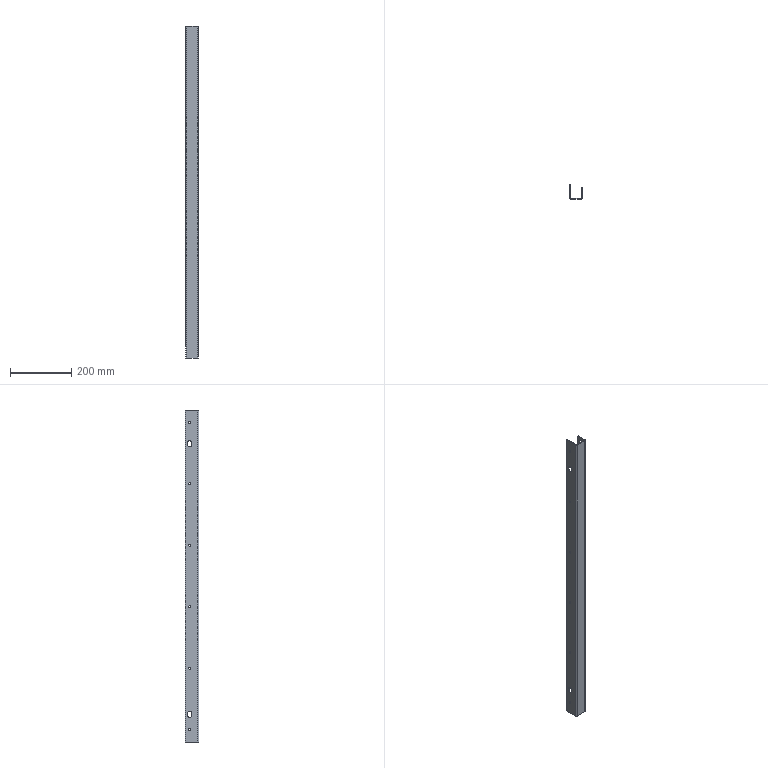Part | STEP file | 5.11.8.01.1033.1 Bracket(Right) | 1 solid | 200 faces | box 42 x 45 x 1080 mm | volume 235963 mm3 | cylinder 100 | plane 100 | commonest cylinder face diameters 9 x64 13 x16 7 x14 23 x4 3 x2